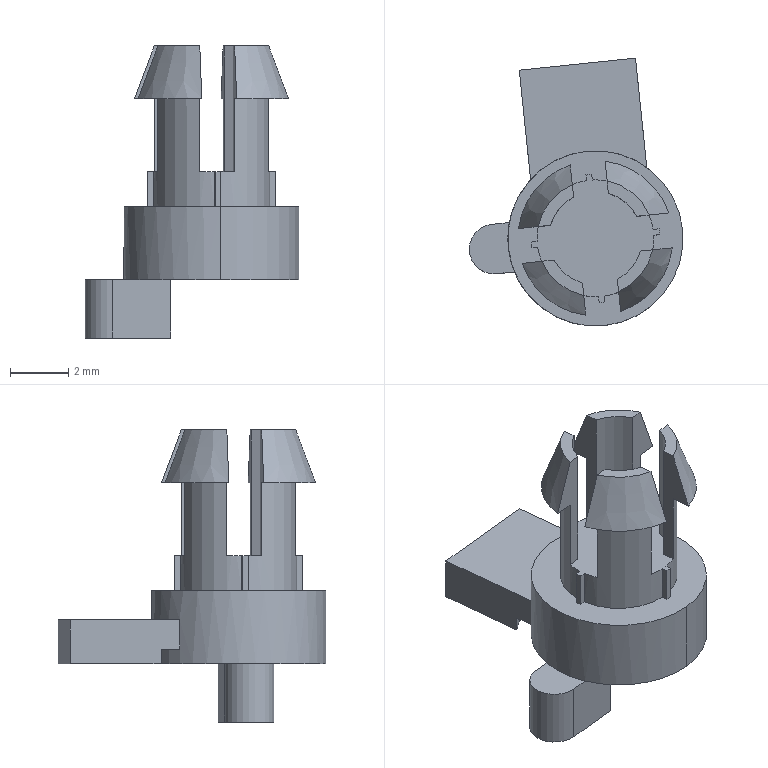Part | STEP file | 1 solid | 64 faces | box 7.319 x 9.174 x 10 mm | volume 108.816 mm3 | plane 44 | cylinder 16 | cone 4 | commonest cylinder face diameters 3.2 x4 4 x4 4.4 x4 6 x2 1.7 x1 7 x1